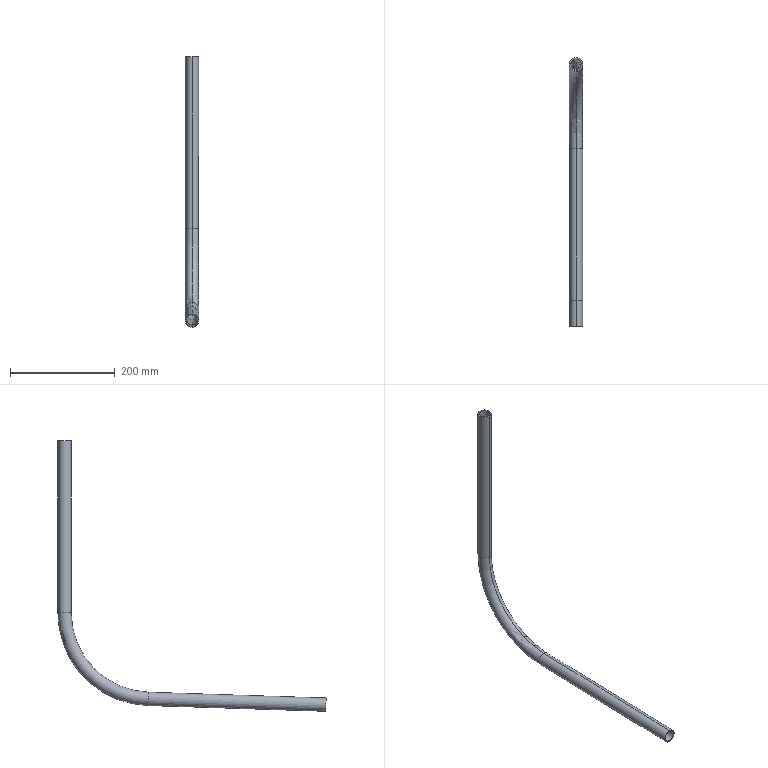Part | STEP file | 31E-01141WG10 | 1 solid | 17 faces | box 25.4 x 512.578 x 517.132 mm | volume 179398 mm3 | cylinder 10 | torus 4 | plane 3 | commonest cylinder face diameters 19.8 x4 25.4 x4 22.2 x2
STEP:
#1=CARTESIAN_POINT('',(0.,0.4122,-12.693));
#2=VERTEX_POINT('',#1);
#3=CARTESIAN_POINT('',(0.,340.233,-1.658));
#4=VERTEX_POINT('',#3);
#5=CARTESIAN_POINT('',(0.,170.323,-7.176));
#6=DIRECTION('',(0.,0.9995,0.03246));
#7=VECTOR('',#6,1.);
#8=LINE('',#5,#7);
#9=EDGE_CURVE('',#2,#4,#8,.T.);
#10=ORIENTED_EDGE('',*,*,#9,.F.);
#11=CARTESIAN_POINT('',(0.,-0.4122,12.693));
#12=VERTEX_POINT('',#11);
#13=CARTESIAN_POINT('',(0.,0.,0.));
#14=DIRECTION('',(0.,0.9995,0.03246));
#15=AXIS2_PLACEMENT_3D('',#13,#14,$);
#16=CIRCLE('',#15,12.7);
#17=EDGE_CURVE('',#2,#12,#16,.T.);
#18=ORIENTED_EDGE('',*,*,#17,.T.);
#19=CARTESIAN_POINT('',(0.,339.409,23.729));
#20=VERTEX_POINT('',#19);
#21=CARTESIAN_POINT('',(0.,169.498,18.211));
#22=DIRECTION('',(0.,0.9995,0.03246));
#23=VECTOR('',#22,1.);
#24=LINE('',#21,#23);
#25=EDGE_CURVE('',#12,#20,#24,.T.);
#26=ORIENTED_EDGE('',*,*,#25,.T.);
#27=CARTESIAN_POINT('',(0.,339.821,11.036));
#28=DIRECTION('',(0.,0.9995,0.03246));
#29=AXIS2_PLACEMENT_3D('',#27,#28,$);
#30=CIRCLE('',#29,12.7);
#31=EDGE_CURVE('',#4,#20,#30,.T.);
#32=ORIENTED_EDGE('',*,*,#31,.F.);
#33=EDGE_LOOP('',(#10,#18,#26,#32));
#34=FACE_OUTER_BOUND('',#33,.T.);
#35=CARTESIAN_POINT('',(0.,169.91,5.518));
#36=DIRECTION('',(0.,0.9995,0.03246));
#37=DIRECTION('',(0.,0.03246,-0.9995));
#38=AXIS2_PLACEMENT_3D('',#35,#36,#37);
#39=CYLINDRICAL_SURFACE('',#38,12.7);
#40=ADVANCED_FACE('',(#34),#39,.T.);
#41=ORIENTED_EDGE('',*,*,#25,.F.);
#42=CARTESIAN_POINT('',(0.,0.,0.));
#43=DIRECTION('',(0.,0.9995,0.03246));
#44=AXIS2_PLACEMENT_3D('',#42,#43,$);
#45=CIRCLE('',#44,12.7);
#46=EDGE_CURVE('',#12,#2,#45,.T.);
#47=ORIENTED_EDGE('',*,*,#46,.T.);
#48=ORIENTED_EDGE('',*,*,#9,.T.);
#49=CARTESIAN_POINT('',(0.,339.821,11.036));
#50=DIRECTION('',(0.,0.9995,0.03246));
#51=AXIS2_PLACEMENT_3D('',#49,#50,$);
#52=CIRCLE('',#51,12.7);
#53=EDGE_CURVE('',#20,#4,#52,.T.);
#54=ORIENTED_EDGE('',*,*,#53,.F.);
#55=EDGE_LOOP('',(#41,#47,#48,#54));
#56=FACE_OUTER_BOUND('',#55,.T.);
#57=CARTESIAN_POINT('',(0.,169.91,5.518));
#58=DIRECTION('',(0.,0.9995,0.03246));
#59=DIRECTION('',(0.,-0.03246,0.9995));
#60=AXIS2_PLACEMENT_3D('',#57,#58,#59);
#61=CYLINDRICAL_SURFACE('',#60,12.7);
#62=ADVANCED_FACE('',(#56),#61,.T.);
#63=CARTESIAN_POINT('',(0.,512.165,175.949));
#64=VERTEX_POINT('',#63);
#65=CARTESIAN_POINT('',(0.,334.465,175.949));
#66=DIRECTION('',(1.,0.,0.));
#67=AXIS2_PLACEMENT_3D('',#65,#66,$);
#68=CIRCLE('',#67,177.7);
#69=EDGE_CURVE('',#4,#64,#68,.T.);
#70=ORIENTED_EDGE('',*,*,#69,.F.);
#71=ORIENTED_EDGE('',*,*,#31,.T.);
#72=CARTESIAN_POINT('',(0.,486.765,175.949));
#73=VERTEX_POINT('',#72);
#74=CARTESIAN_POINT('',(0.,334.465,175.949));
#75=DIRECTION('',(1.,0.,0.));
#76=AXIS2_PLACEMENT_3D('',#74,#75,$);
#77=CIRCLE('',#76,152.3);
#78=EDGE_CURVE('',#20,#73,#77,.T.);
#79=ORIENTED_EDGE('',*,*,#78,.T.);
#80=CARTESIAN_POINT('',(0.,499.465,175.949));
#81=DIRECTION('',(0.,0.,-1.));
#82=AXIS2_PLACEMENT_3D('',#80,#81,$);
#83=CIRCLE('',#82,12.7);
#84=EDGE_CURVE('',#64,#73,#83,.F.);
#85=ORIENTED_EDGE('',*,*,#84,.F.);
#86=EDGE_LOOP('',(#70,#71,#79,#85));
#87=FACE_OUTER_BOUND('',#86,.T.);
#88=CARTESIAN_POINT('',(0.,334.465,175.949));
#89=DIRECTION('',(1.,0.,0.));
#90=DIRECTION('',(0.,0.03246,-0.9995));
#91=AXIS2_PLACEMENT_3D('',#88,#89,#90);
#92=TOROIDAL_SURFACE('',#91,165.,12.7);
#93=ADVANCED_FACE('',(#87),#92,.T.);
#94=ORIENTED_EDGE('',*,*,#78,.F.);
#95=ORIENTED_EDGE('',*,*,#53,.T.);
#96=ORIENTED_EDGE('',*,*,#69,.T.);
#97=CARTESIAN_POINT('',(0.,499.465,175.949));
#98=DIRECTION('',(0.,0.,-1.));
#99=AXIS2_PLACEMENT_3D('',#97,#98,$);
#100=CIRCLE('',#99,12.7);
#101=EDGE_CURVE('',#73,#64,#100,.F.);
#102=ORIENTED_EDGE('',*,*,#101,.F.);
#103=EDGE_LOOP('',(#94,#95,#96,#102));
#104=FACE_OUTER_BOUND('',#103,.T.);
#105=CARTESIAN_POINT('',(0.,334.465,175.949));
#106=DIRECTION('',(1.,0.,0.));
#107=DIRECTION('',(0.,0.03246,-0.9995));
#108=AXIS2_PLACEMENT_3D('',#105,#106,#107);
#109=TOROIDAL_SURFACE('',#108,165.,12.7);
#110=ADVANCED_FACE('',(#104),#109,.T.);
#111=CARTESIAN_POINT('',(0.,512.165,504.439));
#112=VERTEX_POINT('',#111);
#113=CARTESIAN_POINT('',(0.,512.165,340.194));
#114=DIRECTION('',(0.,0.,1.));
#115=VECTOR('',#114,1.);
#116=LINE('',#113,#115);
#117=EDGE_CURVE('',#64,#112,#116,.T.);
#118=ORIENTED_EDGE('',*,*,#117,.F.);
#119=ORIENTED_EDGE('',*,*,#84,.T.);
#120=CARTESIAN_POINT('',(0.,486.765,504.439));
#121=VERTEX_POINT('',#120);
#122=CARTESIAN_POINT('',(0.,486.765,340.194));
#123=DIRECTION('',(0.,0.,1.));
#124=VECTOR('',#123,1.);
#125=LINE('',#122,#124);
#126=EDGE_CURVE('',#73,#121,#125,.T.);
#127=ORIENTED_EDGE('',*,*,#126,.T.);
#128=CARTESIAN_POINT('',(0.,499.465,504.439));
#129=DIRECTION('',(0.,0.,1.));
#130=AXIS2_PLACEMENT_3D('',#128,#129,$);
#131=CIRCLE('',#130,12.7);
#132=EDGE_CURVE('',#112,#121,#131,.T.);
#133=ORIENTED_EDGE('',*,*,#132,.F.);
#134=EDGE_LOOP('',(#118,#119,#127,#133));
#135=FACE_OUTER_BOUND('',#134,.T.);
#136=CARTESIAN_POINT('',(0.,499.465,340.194));
#137=DIRECTION('',(0.,0.,1.));
#138=DIRECTION('',(0.,1.,0.));
#139=AXIS2_PLACEMENT_3D('',#136,#137,#138);
#140=CYLINDRICAL_SURFACE('',#139,12.7);
#141=ADVANCED_FACE('',(#135),#140,.T.);
#142=ORIENTED_EDGE('',*,*,#126,.F.);
#143=ORIENTED_EDGE('',*,*,#101,.T.);
#144=ORIENTED_EDGE('',*,*,#117,.T.);
#145=CARTESIAN_POINT('',(0.,499.465,504.439));
#146=DIRECTION('',(0.,0.,1.));
#147=AXIS2_PLACEMENT_3D('',#145,#146,$);
#148=CIRCLE('',#147,12.7);
#149=EDGE_CURVE('',#121,#112,#148,.T.);
#150=ORIENTED_EDGE('',*,*,#149,.F.);
#151=EDGE_LOOP('',(#142,#143,#144,#150));
#152=FACE_OUTER_BOUND('',#151,.T.);
#153=CARTESIAN_POINT('',(0.,499.465,340.194));
#154=DIRECTION('',(0.,0.,1.));
#155=DIRECTION('',(0.,-1.,0.));
#156=AXIS2_PLACEMENT_3D('',#153,#154,#155);
#157=CYLINDRICAL_SURFACE('',#156,12.7);
#158=ADVANCED_FACE('',(#152),#157,.T.);
#159=CARTESIAN_POINT('',(0.,489.565,175.949));
#160=VERTEX_POINT('',#159);
#161=CARTESIAN_POINT('',(0.,509.365,175.949));
#162=VERTEX_POINT('',#161);
#163=CARTESIAN_POINT('',(0.,499.465,175.949));
#164=DIRECTION('',(0.,0.,-1.));
#165=AXIS2_PLACEMENT_3D('',#163,#164,$);
#166=CIRCLE('',#165,9.9);
#167=EDGE_CURVE('',#160,#162,#166,.F.);
#168=ORIENTED_EDGE('',*,*,#167,.T.);
#169=CARTESIAN_POINT('',(0.,340.142,1.141));
#170=VERTEX_POINT('',#169);
#171=CARTESIAN_POINT('',(0.,334.465,175.949));
#172=DIRECTION('',(1.,0.,0.));
#173=AXIS2_PLACEMENT_3D('',#171,#172,$);
#174=CIRCLE('',#173,174.9);
#175=EDGE_CURVE('',#170,#162,#174,.T.);
#176=ORIENTED_EDGE('',*,*,#175,.F.);
#177=CARTESIAN_POINT('',(0.,339.5,20.93));
#178=VERTEX_POINT('',#177);
#179=CARTESIAN_POINT('',(0.,339.821,11.036));
#180=DIRECTION('',(0.,-0.9995,-0.03246));
#181=AXIS2_PLACEMENT_3D('',#179,#180,$);
#182=CIRCLE('',#181,9.9);
#183=EDGE_CURVE('',#178,#170,#182,.F.);
#184=ORIENTED_EDGE('',*,*,#183,.F.);
#185=CARTESIAN_POINT('',(0.,334.465,175.949));
#186=DIRECTION('',(1.,0.,0.));
#187=AXIS2_PLACEMENT_3D('',#185,#186,$);
#188=CIRCLE('',#187,155.1);
#189=EDGE_CURVE('',#178,#160,#188,.T.);
#190=ORIENTED_EDGE('',*,*,#189,.T.);
#191=EDGE_LOOP('',(#168,#176,#184,#190));
#192=FACE_OUTER_BOUND('',#191,.T.);
#193=CARTESIAN_POINT('',(0.,334.465,175.949));
#194=DIRECTION('',(1.,0.,0.));
#195=DIRECTION('',(0.,0.03246,-0.9995));
#196=AXIS2_PLACEMENT_3D('',#193,#194,#195);
#197=TOROIDAL_SURFACE('',#196,165.,9.9);
#198=ADVANCED_FACE('',(#192),#197,.F.);
#199=CARTESIAN_POINT('',(0.,499.465,175.949));
#200=DIRECTION('',(0.,0.,-1.));
#201=AXIS2_PLACEMENT_3D('',#199,#200,$);
#202=CIRCLE('',#201,9.9);
#203=EDGE_CURVE('',#162,#160,#202,.F.);
#204=ORIENTED_EDGE('',*,*,#203,.T.);
#205=ORIENTED_EDGE('',*,*,#189,.F.);
#206=CARTESIAN_POINT('',(0.,339.821,11.036));
#207=DIRECTION('',(0.,-0.9995,-0.03246));
#208=AXIS2_PLACEMENT_3D('',#206,#207,$);
#209=CIRCLE('',#208,9.9);
#210=EDGE_CURVE('',#170,#178,#209,.F.);
#211=ORIENTED_EDGE('',*,*,#210,.F.);
#212=ORIENTED_EDGE('',*,*,#175,.T.);
#213=EDGE_LOOP('',(#204,#205,#211,#212));
#214=FACE_OUTER_BOUND('',#213,.T.);
#215=CARTESIAN_POINT('',(0.,334.465,175.949));
#216=DIRECTION('',(1.,0.,0.));
#217=DIRECTION('',(0.,0.03246,-0.9995));
#218=AXIS2_PLACEMENT_3D('',#215,#216,#217);
#219=TOROIDAL_SURFACE('',#218,165.,9.9);
#220=ADVANCED_FACE('',(#214),#219,.F.);
#221=ORIENTED_EDGE('',*,*,#132,.T.);
#222=ORIENTED_EDGE('',*,*,#149,.T.);
#223=EDGE_LOOP('',(#221,#222));
#224=FACE_OUTER_BOUND('',#223,.T.);
#225=CARTESIAN_POINT('',(0.,489.565,504.439));
#226=VERTEX_POINT('',#225);
#227=CARTESIAN_POINT('',(0.,509.365,504.439));
#228=VERTEX_POINT('',#227);
#229=CARTESIAN_POINT('',(0.,499.465,504.439));
#230=DIRECTION('',(0.,0.,-1.));
#231=AXIS2_PLACEMENT_3D('',#229,#230,$);
#232=CIRCLE('',#231,9.9);
#233=EDGE_CURVE('',#226,#228,#232,.F.);
#234=ORIENTED_EDGE('',*,*,#233,.F.);
#235=CARTESIAN_POINT('',(0.,499.465,504.439));
#236=DIRECTION('',(0.,0.,-1.));
#237=AXIS2_PLACEMENT_3D('',#235,#236,$);
#238=CIRCLE('',#237,9.9);
#239=EDGE_CURVE('',#228,#226,#238,.F.);
#240=ORIENTED_EDGE('',*,*,#239,.F.);
#241=EDGE_LOOP('',(#234,#240));
#242=FACE_BOUND('',#241,.T.);
#243=CARTESIAN_POINT('',(0.,499.465,504.439));
#244=DIRECTION('',(0.,0.,-1.));
#245=DIRECTION('',(0.,1.,0.));
#246=AXIS2_PLACEMENT_3D('',#243,#244,#245);
#247=PLANE('',#246);
#248=ADVANCED_FACE('',(#224,#242),#247,.F.);
#249=ORIENTED_EDGE('',*,*,#233,.T.);
#250=CARTESIAN_POINT('',(0.,509.365,340.194));
#251=DIRECTION('',(0.,0.,1.));
#252=VECTOR('',#251,1.);
#253=LINE('',#250,#252);
#254=EDGE_CURVE('',#162,#228,#253,.T.);
#255=ORIENTED_EDGE('',*,*,#254,.F.);
#256=ORIENTED_EDGE('',*,*,#167,.F.);
#257=CARTESIAN_POINT('',(0.,489.565,340.194));
#258=DIRECTION('',(0.,0.,1.));
#259=VECTOR('',#258,1.);
#260=LINE('',#257,#259);
#261=EDGE_CURVE('',#160,#226,#260,.T.);
#262=ORIENTED_EDGE('',*,*,#261,.T.);
#263=EDGE_LOOP('',(#249,#255,#256,#262));
#264=FACE_OUTER_BOUND('',#263,.T.);
#265=CARTESIAN_POINT('',(0.,499.465,340.194));
#266=DIRECTION('',(0.,0.,1.));
#267=DIRECTION('',(0.,-1.,0.));
#268=AXIS2_PLACEMENT_3D('',#265,#266,#267);
#269=CYLINDRICAL_SURFACE('',#268,9.9);
#270=ADVANCED_FACE('',(#264),#269,.F.);
#271=ORIENTED_EDGE('',*,*,#239,.T.);
#272=ORIENTED_EDGE('',*,*,#261,.F.);
#273=ORIENTED_EDGE('',*,*,#203,.F.);
#274=ORIENTED_EDGE('',*,*,#254,.T.);
#275=EDGE_LOOP('',(#271,#272,#273,#274));
#276=FACE_OUTER_BOUND('',#275,.T.);
#277=CARTESIAN_POINT('',(0.,499.465,340.194));
#278=DIRECTION('',(0.,0.,1.));
#279=DIRECTION('',(0.,1.,0.));
#280=AXIS2_PLACEMENT_3D('',#277,#278,#279);
#281=CYLINDRICAL_SURFACE('',#280,9.9);
#282=ADVANCED_FACE('',(#276),#281,.F.);
#283=CARTESIAN_POINT('',(0.,49.652,11.518));
#284=VERTEX_POINT('',#283);
#285=CARTESIAN_POINT('',(0.,50.295,-8.272));
#286=VERTEX_POINT('',#285);
#287=CARTESIAN_POINT('',(0.,49.974,1.623));
#288=DIRECTION('',(0.,0.9995,0.03246));
#289=AXIS2_PLACEMENT_3D('',#287,#288,$);
#290=CIRCLE('',#289,9.9);
#291=EDGE_CURVE('',#284,#286,#290,.F.);
#292=ORIENTED_EDGE('',*,*,#291,.T.);
#293=CARTESIAN_POINT('',(0.,170.232,-4.377));
#294=DIRECTION('',(0.,0.9995,0.03246));
#295=VECTOR('',#294,1.);
#296=LINE('',#293,#295);
#297=EDGE_CURVE('',#286,#170,#296,.T.);
#298=ORIENTED_EDGE('',*,*,#297,.T.);
#299=ORIENTED_EDGE('',*,*,#210,.T.);
#300=CARTESIAN_POINT('',(0.,169.589,15.413));
#301=DIRECTION('',(0.,0.9995,0.03246));
#302=VECTOR('',#301,1.);
#303=LINE('',#300,#302);
#304=EDGE_CURVE('',#284,#178,#303,.T.);
#305=ORIENTED_EDGE('',*,*,#304,.F.);
#306=EDGE_LOOP('',(#292,#298,#299,#305));
#307=FACE_OUTER_BOUND('',#306,.T.);
#308=CARTESIAN_POINT('',(0.,169.91,5.518));
#309=DIRECTION('',(0.,0.9995,0.03246));
#310=DIRECTION('',(0.,0.03246,-0.9995));
#311=AXIS2_PLACEMENT_3D('',#308,#309,#310);
#312=CYLINDRICAL_SURFACE('',#311,9.9);
#313=ADVANCED_FACE('',(#307),#312,.F.);
#314=CARTESIAN_POINT('',(0.,49.974,1.623));
#315=DIRECTION('',(0.,0.9995,0.03246));
#316=AXIS2_PLACEMENT_3D('',#314,#315,$);
#317=CIRCLE('',#316,9.9);
#318=EDGE_CURVE('',#286,#284,#317,.F.);
#319=ORIENTED_EDGE('',*,*,#318,.T.);
#320=ORIENTED_EDGE('',*,*,#304,.T.);
#321=ORIENTED_EDGE('',*,*,#183,.T.);
#322=ORIENTED_EDGE('',*,*,#297,.F.);
#323=EDGE_LOOP('',(#319,#320,#321,#322));
#324=FACE_OUTER_BOUND('',#323,.T.);
#325=CARTESIAN_POINT('',(0.,169.91,5.518));
#326=DIRECTION('',(0.,0.9995,0.03246));
#327=DIRECTION('',(0.,-0.03246,0.9995));
#328=AXIS2_PLACEMENT_3D('',#325,#326,#327);
#329=CYLINDRICAL_SURFACE('',#328,9.9);
#330=ADVANCED_FACE('',(#324),#329,.F.);
#331=ORIENTED_EDGE('',*,*,#46,.F.);
#332=ORIENTED_EDGE('',*,*,#17,.F.);
#333=EDGE_LOOP('',(#331,#332));
#334=FACE_OUTER_BOUND('',#333,.T.);
#335=CARTESIAN_POINT('',(-11.1,0.,0.));
#336=VERTEX_POINT('',#335);
#337=CARTESIAN_POINT('',(11.1,0.,0.));
#338=VERTEX_POINT('',#337);
#339=CARTESIAN_POINT('',(0.,0.,0.));
#340=DIRECTION('',(0.,0.9995,0.03246));
#341=AXIS2_PLACEMENT_3D('',#339,#340,$);
#342=CIRCLE('',#341,11.1);
#343=EDGE_CURVE('',#336,#338,#342,.F.);
#344=ORIENTED_EDGE('',*,*,#343,.F.);
#345=CARTESIAN_POINT('',(0.,0.,0.));
#346=DIRECTION('',(0.,0.9995,0.03246));
#347=AXIS2_PLACEMENT_3D('',#345,#346,$);
#348=CIRCLE('',#347,11.1);
#349=EDGE_CURVE('',#338,#336,#348,.F.);
#350=ORIENTED_EDGE('',*,*,#349,.F.);
#351=EDGE_LOOP('',(#344,#350));
#352=FACE_BOUND('',#351,.T.);
#353=CARTESIAN_POINT('',(0.,0.,0.));
#354=DIRECTION('',(0.,0.9995,0.03246));
#355=DIRECTION('',(0.,0.03246,-0.9995));
#356=AXIS2_PLACEMENT_3D('',#353,#354,#355);
#357=PLANE('',#356);
#358=ADVANCED_FACE('',(#334,#352),#357,.F.);
#359=CARTESIAN_POINT('',(11.1,49.974,1.623));
#360=VERTEX_POINT('',#359);
#361=CARTESIAN_POINT('',(11.1,24.987,0.8114));
#362=DIRECTION('',(0.,-0.9995,-0.03246));
#363=VECTOR('',#362,1.);
#364=LINE('',#361,#363);
#365=EDGE_CURVE('',#338,#360,#364,.F.);
#366=ORIENTED_EDGE('',*,*,#365,.F.);
#367=ORIENTED_EDGE('',*,*,#349,.T.);
#368=CARTESIAN_POINT('',(-11.1,49.974,1.623));
#369=VERTEX_POINT('',#368);
#370=CARTESIAN_POINT('',(-11.1,24.987,0.8114));
#371=DIRECTION('',(0.,-0.9995,-0.03246));
#372=VECTOR('',#371,1.);
#373=LINE('',#370,#372);
#374=EDGE_CURVE('',#336,#369,#373,.F.);
#375=ORIENTED_EDGE('',*,*,#374,.T.);
#376=CARTESIAN_POINT('',(0.,49.974,1.623));
#377=DIRECTION('',(0.,-0.9995,-0.03246));
#378=AXIS2_PLACEMENT_3D('',#376,#377,$);
#379=CIRCLE('',#378,11.1);
#380=EDGE_CURVE('',#360,#369,#379,.T.);
#381=ORIENTED_EDGE('',*,*,#380,.F.);
#382=EDGE_LOOP('',(#366,#367,#375,#381));
#383=FACE_OUTER_BOUND('',#382,.T.);
#384=CARTESIAN_POINT('',(0.,24.987,0.8114));
#385=DIRECTION('',(0.,-0.9995,-0.03246));
#386=DIRECTION('',(1.,0.,0.));
#387=AXIS2_PLACEMENT_3D('',#384,#385,#386);
#388=CYLINDRICAL_SURFACE('',#387,11.1);
#389=ADVANCED_FACE('',(#383),#388,.F.);
#390=ORIENTED_EDGE('',*,*,#374,.F.);
#391=ORIENTED_EDGE('',*,*,#343,.T.);
#392=ORIENTED_EDGE('',*,*,#365,.T.);
#393=CARTESIAN_POINT('',(0.,49.974,1.623));
#394=DIRECTION('',(0.,-0.9995,-0.03246));
#395=AXIS2_PLACEMENT_3D('',#393,#394,$);
#396=CIRCLE('',#395,11.1);
#397=EDGE_CURVE('',#369,#360,#396,.T.);
#398=ORIENTED_EDGE('',*,*,#397,.F.);
#399=EDGE_LOOP('',(#390,#391,#392,#398));
#400=FACE_OUTER_BOUND('',#399,.T.);
#401=ADVANCED_FACE('',(#400),#388,.F.);
#402=ORIENTED_EDGE('',*,*,#380,.T.);
#403=ORIENTED_EDGE('',*,*,#397,.T.);
#404=EDGE_LOOP('',(#402,#403));
#405=FACE_OUTER_BOUND('',#404,.T.);
#406=ORIENTED_EDGE('',*,*,#318,.F.);
#407=ORIENTED_EDGE('',*,*,#291,.F.);
#408=EDGE_LOOP('',(#406,#407));
#409=FACE_BOUND('',#408,.T.);
#410=CARTESIAN_POINT('',(0.,49.974,1.623));
#411=DIRECTION('',(0.,-0.9995,-0.03246));
#412=DIRECTION('',(1.,0.,0.));
#413=AXIS2_PLACEMENT_3D('',#410,#411,#412);
#414=PLANE('',#413);
#415=ADVANCED_FACE('',(#405,#409),#414,.T.);
#416=CLOSED_SHELL('',(#40,#62,#93,#110,#141,#158,#198,#220,#248,#270,#282,#313,#330,#358,#389,#401,#415));
#417=MANIFOLD_SOLID_BREP('',#416);
#418=(LENGTH_UNIT()NAMED_UNIT(*)SI_UNIT(.MILLI.,.METRE.));
#419=UNCERTAINTY_MEASURE_WITH_UNIT(LENGTH_MEASURE(0.005),#418,'','');
#420=(NAMED_UNIT(*)PLANE_ANGLE_UNIT()SI_UNIT($,.RADIAN.));
#421=(NAMED_UNIT(*)SI_UNIT($,.STERADIAN.)SOLID_ANGLE_UNIT());
#422=(GEOMETRIC_REPRESENTATION_CONTEXT(3)GLOBAL_UNCERTAINTY_ASSIGNED_CONTEXT((#419))GLOBAL_UNIT_ASSIGNED_CONTEXT((#418,#420,#421))REPRESENTATION_CONTEXT('',''));
#423=ADVANCED_BREP_SHAPE_REPRESENTATION('',(#417),#422);